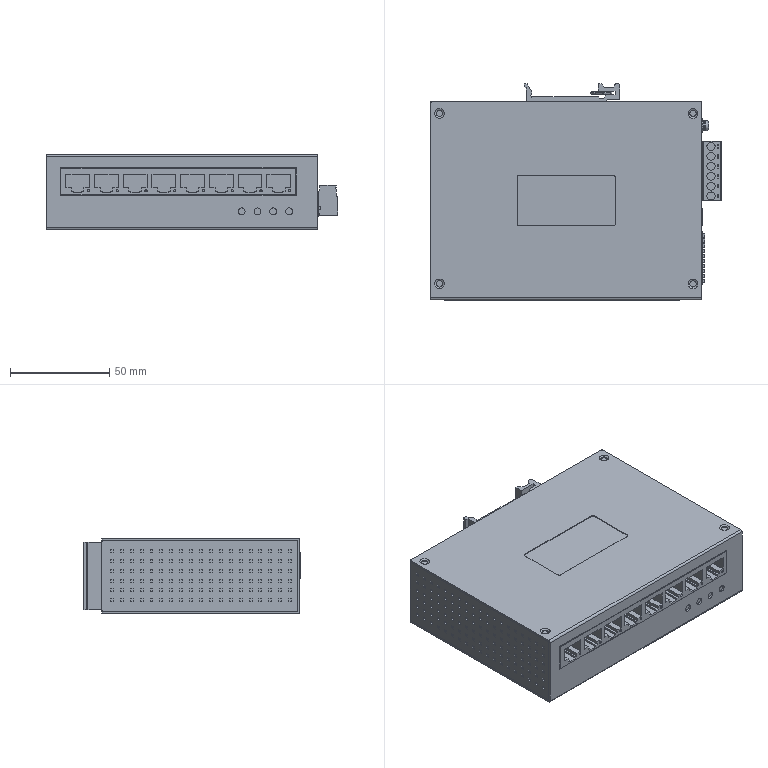Part | SolidWorks | features BaseBody 9 | 9 solids | 1825 faces | box 146.9 x 109.2 x 38 mm | volume 517225 mm3 | plane 1477 | cylinder 270 | cone 43 | torus 17 | sphere 10 | spline 8 | commonest cylinder face diameters 3 x44 2 x26 1.2 x24 0.6 x21 0.2 x20 0.4 x17